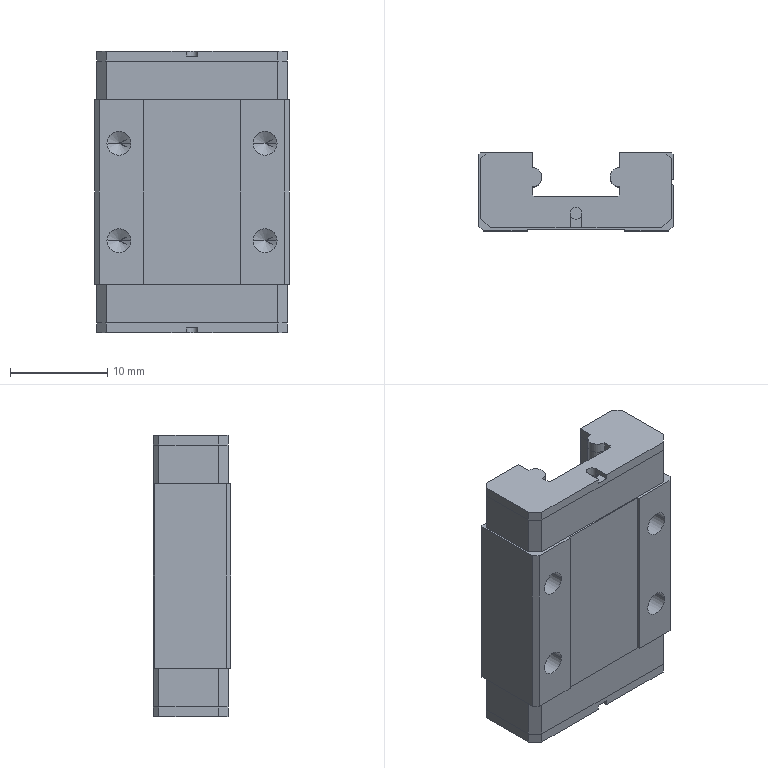Part | SolidWorks | features BaseBody 5 | 5 solids | 141 faces | box 20 x 8 x 28.9 mm | volume 3330 mm3 | plane 101 | cylinder 32 | cone 8 | commonest cylinder face diameters 2 x15 1.2 x8 2.459 x8 0.6 x1